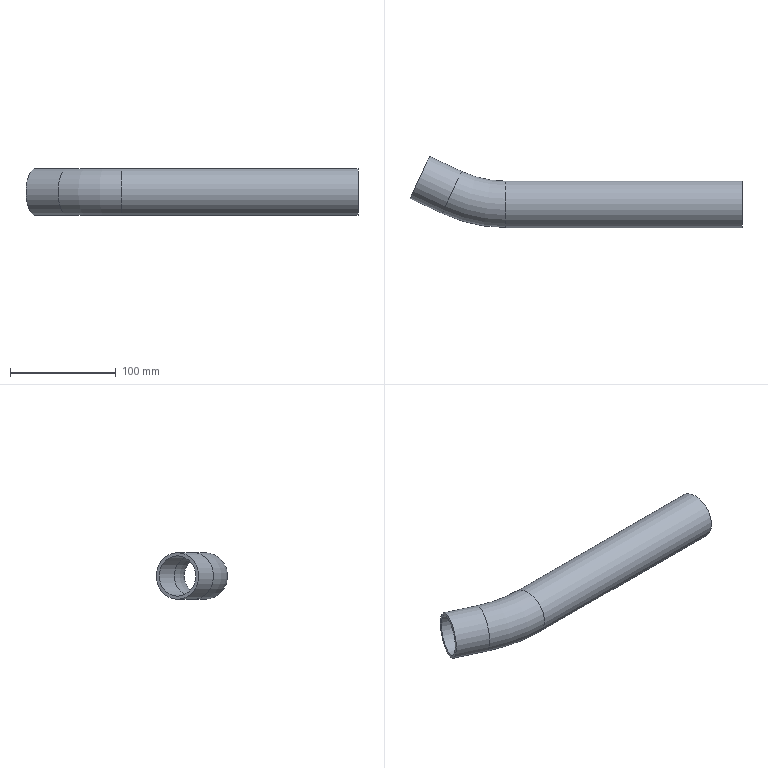Part | STEP file | 6151201WA | 1 solid | 8 faces | box 313.697 x 67.391 x 44.1 mm | volume 119753 mm3 | cylinder 4 | torus 2 | plane 2 | commonest cylinder face diameters 38.1 x2 44.1 x2
STEP:
#1=CARTESIAN_POINT('',(-274.111,11.243,-22.05));
#2=VERTEX_POINT('',#1);
#3=CARTESIAN_POINT('',(-274.111,11.243,0.));
#4=DIRECTION('',(0.9063,-0.4226,0.));
#5=DIRECTION('',(0.,0.,-1.));
#6=AXIS2_PLACEMENT_3D('',#3,#4,#5);
#7=CIRCLE('',#6,22.05);
#8=EDGE_CURVE('',#2,#2,#7,.T.);
#9=ORIENTED_EDGE('',*,*,#8,.F.);
#10=EDGE_LOOP('',(#9));
#11=FACE_OUTER_BOUND('',#10,.T.);
#12=CARTESIAN_POINT('',(-304.378,25.357,-22.05));
#13=VERTEX_POINT('',#12);
#14=CARTESIAN_POINT('',(-304.378,25.357,0.));
#15=DIRECTION('',(0.9063,-0.4226,0.));
#16=DIRECTION('',(0.,0.,-1.));
#17=AXIS2_PLACEMENT_3D('',#14,#15,#16);
#18=CIRCLE('',#17,22.05);
#19=EDGE_CURVE('',#13,#13,#18,.T.);
#20=ORIENTED_EDGE('',*,*,#19,.T.);
#21=EDGE_LOOP('',(#20));
#22=FACE_OUTER_BOUND('',#21,.T.);
#23=CARTESIAN_POINT('',(-274.111,11.243,0.));
#24=DIRECTION('',(-0.9063,0.4226,0.));
#25=DIRECTION('',(-0.4226,-0.9063,0.));
#26=AXIS2_PLACEMENT_3D('',#23,#24,#25);
#27=CYLINDRICAL_SURFACE('',#26,22.05);
#28=ADVANCED_FACE('',(#11,#22),#27,.T.);
#29=CARTESIAN_POINT('',(-274.111,11.243,-19.05));
#30=VERTEX_POINT('',#29);
#31=CARTESIAN_POINT('',(-274.111,11.243,0.));
#32=DIRECTION('',(0.9063,-0.4226,0.));
#33=DIRECTION('',(0.,0.,-1.));
#34=AXIS2_PLACEMENT_3D('',#31,#32,#33);
#35=CIRCLE('',#34,19.05);
#36=EDGE_CURVE('',#30,#30,#35,.T.);
#37=ORIENTED_EDGE('',*,*,#36,.T.);
#38=EDGE_LOOP('',(#37));
#39=FACE_OUTER_BOUND('',#38,.T.);
#40=CARTESIAN_POINT('',(-304.378,25.357,-19.05));
#41=VERTEX_POINT('',#40);
#42=CARTESIAN_POINT('',(-304.378,25.357,0.));
#43=DIRECTION('',(0.9063,-0.4226,0.));
#44=DIRECTION('',(0.,0.,-1.));
#45=AXIS2_PLACEMENT_3D('',#42,#43,#44);
#46=CIRCLE('',#45,19.05);
#47=EDGE_CURVE('',#41,#41,#46,.T.);
#48=ORIENTED_EDGE('',*,*,#47,.F.);
#49=EDGE_LOOP('',(#48));
#50=FACE_OUTER_BOUND('',#49,.T.);
#51=CARTESIAN_POINT('',(-274.111,11.243,0.));
#52=DIRECTION('',(-0.9063,0.4226,0.));
#53=DIRECTION('',(-0.4226,-0.9063,0.));
#54=AXIS2_PLACEMENT_3D('',#51,#52,#53);
#55=CYLINDRICAL_SURFACE('',#54,19.05);
#56=ADVANCED_FACE('',(#39,#50),#55,.F.);
#57=CARTESIAN_POINT('',(-223.397,0.,-22.05));
#58=VERTEX_POINT('',#57);
#59=CARTESIAN_POINT('',(-223.397,0.,0.));
#60=DIRECTION('',(1.,0.,0.));
#61=DIRECTION('',(0.,0.,-1.));
#62=AXIS2_PLACEMENT_3D('',#59,#60,#61);
#63=CIRCLE('',#62,22.05);
#64=EDGE_CURVE('',#58,#58,#63,.T.);
#65=ORIENTED_EDGE('',*,*,#64,.F.);
#66=EDGE_LOOP('',(#65));
#67=FACE_OUTER_BOUND('',#66,.T.);
#68=ORIENTED_EDGE('',*,*,#8,.T.);
#69=EDGE_LOOP('',(#68));
#70=FACE_OUTER_BOUND('',#69,.T.);
#71=CARTESIAN_POINT('',(-223.397,120.,0.));
#72=DIRECTION('',(0.,0.,-1.));
#73=DIRECTION('',(-1.,0.,0.));
#74=AXIS2_PLACEMENT_3D('',#71,#72,#73);
#75=TOROIDAL_SURFACE('',#74,120.,22.05);
#76=ADVANCED_FACE('',(#67,#70),#75,.T.);
#77=CARTESIAN_POINT('',(-223.397,0.,-19.05));
#78=VERTEX_POINT('',#77);
#79=CARTESIAN_POINT('',(-223.397,0.,0.));
#80=DIRECTION('',(1.,0.,0.));
#81=DIRECTION('',(0.,0.,-1.));
#82=AXIS2_PLACEMENT_3D('',#79,#80,#81);
#83=CIRCLE('',#82,19.05);
#84=EDGE_CURVE('',#78,#78,#83,.T.);
#85=ORIENTED_EDGE('',*,*,#84,.T.);
#86=EDGE_LOOP('',(#85));
#87=FACE_OUTER_BOUND('',#86,.T.);
#88=ORIENTED_EDGE('',*,*,#36,.F.);
#89=EDGE_LOOP('',(#88));
#90=FACE_OUTER_BOUND('',#89,.T.);
#91=CARTESIAN_POINT('',(-223.397,120.,0.));
#92=DIRECTION('',(0.,0.,-1.));
#93=DIRECTION('',(-1.,0.,0.));
#94=AXIS2_PLACEMENT_3D('',#91,#92,#93);
#95=TOROIDAL_SURFACE('',#94,120.,19.05);
#96=ADVANCED_FACE('',(#87,#90),#95,.F.);
#97=ORIENTED_EDGE('',*,*,#84,.F.);
#98=EDGE_LOOP('',(#97));
#99=FACE_OUTER_BOUND('',#98,.T.);
#100=CARTESIAN_POINT('',(0.,0.,-19.05));
#101=VERTEX_POINT('',#100);
#102=CARTESIAN_POINT('',(0.,0.,0.));
#103=DIRECTION('',(1.,0.,0.));
#104=DIRECTION('',(0.,0.,-1.));
#105=AXIS2_PLACEMENT_3D('',#102,#103,#104);
#106=CIRCLE('',#105,19.05);
#107=EDGE_CURVE('',#101,#101,#106,.T.);
#108=ORIENTED_EDGE('',*,*,#107,.T.);
#109=EDGE_LOOP('',(#108));
#110=FACE_OUTER_BOUND('',#109,.T.);
#111=CARTESIAN_POINT('',(-223.397,0.,0.));
#112=DIRECTION('',(1.,0.,0.));
#113=DIRECTION('',(0.,1.,0.));
#114=AXIS2_PLACEMENT_3D('',#111,#112,#113);
#115=CYLINDRICAL_SURFACE('',#114,19.05);
#116=ADVANCED_FACE('',(#99,#110),#115,.F.);
#117=ORIENTED_EDGE('',*,*,#64,.T.);
#118=EDGE_LOOP('',(#117));
#119=FACE_OUTER_BOUND('',#118,.T.);
#120=CARTESIAN_POINT('',(0.,0.,-22.05));
#121=VERTEX_POINT('',#120);
#122=CARTESIAN_POINT('',(0.,0.,0.));
#123=DIRECTION('',(1.,0.,0.));
#124=DIRECTION('',(0.,0.,-1.));
#125=AXIS2_PLACEMENT_3D('',#122,#123,#124);
#126=CIRCLE('',#125,22.05);
#127=EDGE_CURVE('',#121,#121,#126,.T.);
#128=ORIENTED_EDGE('',*,*,#127,.F.);
#129=EDGE_LOOP('',(#128));
#130=FACE_OUTER_BOUND('',#129,.T.);
#131=CARTESIAN_POINT('',(-223.397,0.,0.));
#132=DIRECTION('',(1.,0.,0.));
#133=DIRECTION('',(0.,1.,0.));
#134=AXIS2_PLACEMENT_3D('',#131,#132,#133);
#135=CYLINDRICAL_SURFACE('',#134,22.05);
#136=ADVANCED_FACE('',(#119,#130),#135,.T.);
#137=ORIENTED_EDGE('',*,*,#47,.T.);
#138=EDGE_LOOP('',(#137));
#139=FACE_BOUND('',#138,.T.);
#140=ORIENTED_EDGE('',*,*,#19,.F.);
#141=EDGE_LOOP('',(#140));
#142=FACE_OUTER_BOUND('',#141,.T.);
#143=CARTESIAN_POINT('',(-304.378,25.357,0.));
#144=DIRECTION('',(0.9063,-0.4226,0.));
#145=DIRECTION('',(0.,0.,-1.));
#146=AXIS2_PLACEMENT_3D('',#143,#144,#145);
#147=PLANE('',#146);
#148=ADVANCED_FACE('',(#139,#142),#147,.F.);
#149=ORIENTED_EDGE('',*,*,#107,.F.);
#150=EDGE_LOOP('',(#149));
#151=FACE_BOUND('',#150,.T.);
#152=ORIENTED_EDGE('',*,*,#127,.T.);
#153=EDGE_LOOP('',(#152));
#154=FACE_OUTER_BOUND('',#153,.T.);
#155=CARTESIAN_POINT('',(0.,0.,0.));
#156=DIRECTION('',(1.,0.,0.));
#157=DIRECTION('',(0.,0.,-1.));
#158=AXIS2_PLACEMENT_3D('',#155,#156,#157);
#159=PLANE('',#158);
#160=ADVANCED_FACE('',(#151,#154),#159,.T.);
#161=CLOSED_SHELL('',(#28,#56,#76,#96,#116,#136,#148,#160));
#162=MANIFOLD_SOLID_BREP('',#161);
#163=CARTESIAN_POINT('',(0.,0.,0.));
#164=DIRECTION('',(0.,0.,1.));
#165=DIRECTION('',(1.,0.,0.));
#166=AXIS2_PLACEMENT_3D('',#163,#164,#165);
#167=(LENGTH_UNIT()NAMED_UNIT(*)SI_UNIT(.MILLI.,.METRE.));
#168=UNCERTAINTY_MEASURE_WITH_UNIT(LENGTH_MEASURE(0.00001),#167,'','');
#169=(NAMED_UNIT(*)PLANE_ANGLE_UNIT()SI_UNIT($,.RADIAN.));
#170=(NAMED_UNIT(*)SI_UNIT($,.STERADIAN.)SOLID_ANGLE_UNIT());
#171=(GEOMETRIC_REPRESENTATION_CONTEXT(3)GLOBAL_UNCERTAINTY_ASSIGNED_CONTEXT((#168))GLOBAL_UNIT_ASSIGNED_CONTEXT((#167,#169,#170))REPRESENTATION_CONTEXT('',''));
#172=ADVANCED_BREP_SHAPE_REPRESENTATION('',(#162,#166),#171);